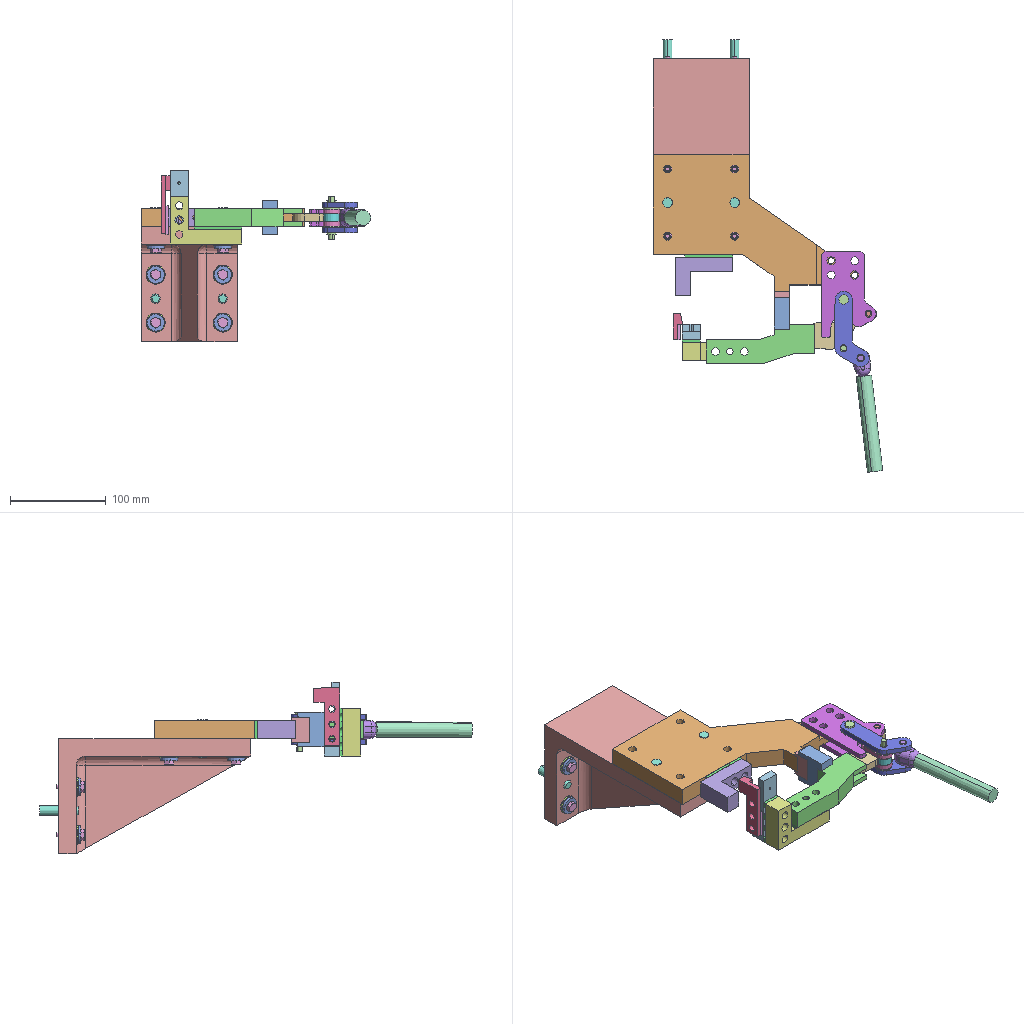Assembly | SolidWorks | 28 different items | 59 placed | box 239 x 451 x 179 mm
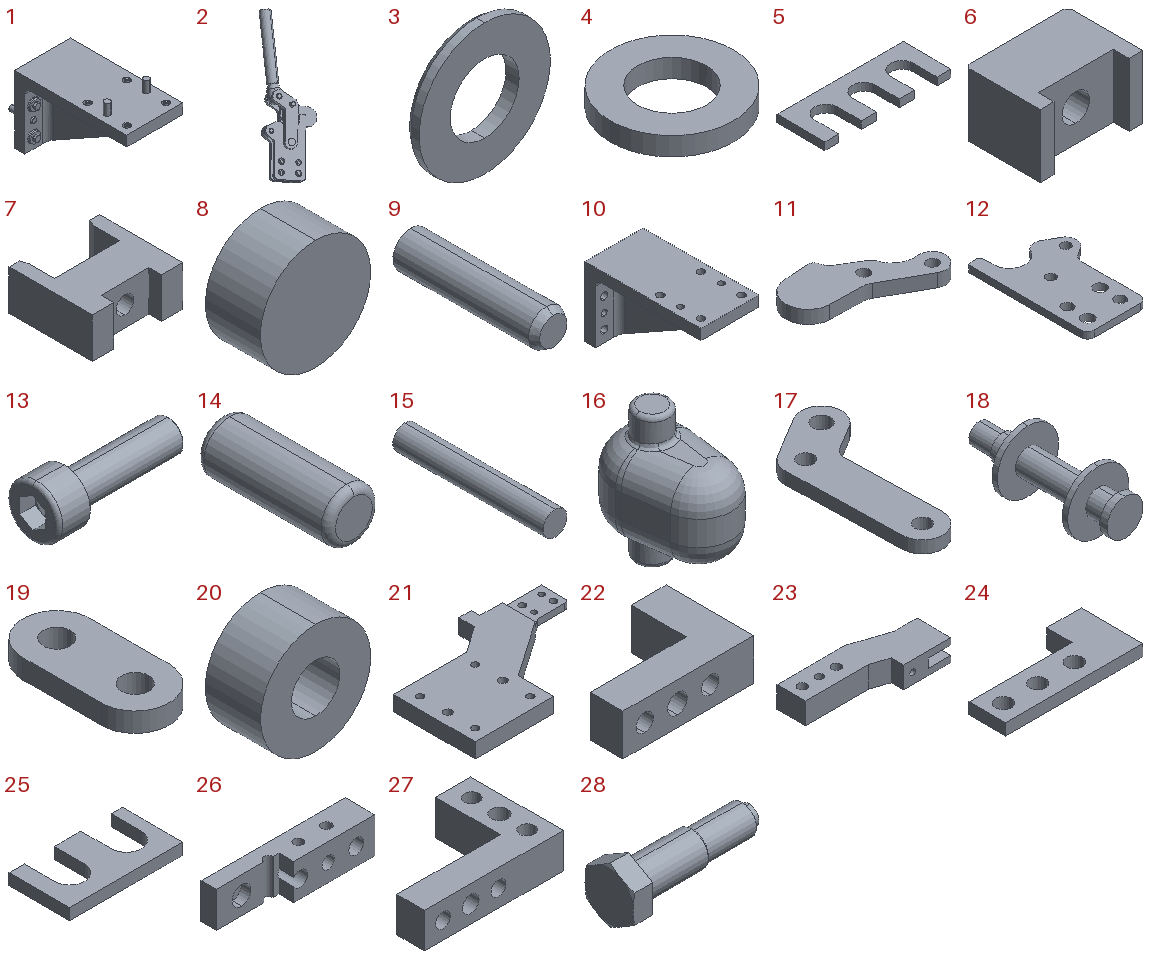Parts list (item | name | quantity | parent item | size | volume | features):
1 | (subassembly) | x1 | - | 100 x 220 x 140 mm | 721947 mm3 | features CompositeCurve 10
2 | (subassembly) | x1 | - | 112.747 x 151.76 x 188.204 mm | 98707 mm3 | features CompositeCurve 3
3 | - | x8 | in 1 | 20 x 2 x 20 mm | 441.839 mm3 | features Chamfer 1, Extrusion 1
4 | - | x8 | in 1 | 18 x 18 x 2.7 mm | 475.009 mm3 | features Extrusion 1
5 | - | x3 | - | 50 x 19 x 3 mm | 1794 mm3 | features Extrusion 1
6 | - | x1 | - | 26 x 19 x 16 mm | 5699 mm3 | features ICE 2, Chamfer 1, Extrusion 1
7 | - | x1 | - | 36 x 33 x 16 mm | 11068 mm3 | features ICE 2, Extrusion 1
8 | - | x1 | - | 10 x 5 x 10 mm | 392.699 mm3 | features Extrusion 1
9 | - | x4 | in 1 | 10 x 40 x 10 mm | 3108 mm3 | features Chamfer 1, Extrusion 1
10 | - | x1 | in 1 | 100 x 200 x 120 mm | 692864 mm3 | features Fillet 2, ICE 2, Extrusion 1, Rib 1
11 | - | x1 | in 2 | 74.927 x 44.837 x 8 mm | 11417 mm3 | features Extrusion 1
12 | - | x2 | in 2 | 56.9 x 90 x 5 mm | 16455 mm3 | features Fillet 2, Extrusion 1
13 | - | x2 | - | 26 x 10 x 10 mm | 958.089 mm3 | features Fillet 2, RevCut 2, Boss 1, Chamfer 1, Cut 1, Extrusion 1, LPattern 1
14 | - | x1 | in 2 | 7 x 18 x 7 mm | 683.885 mm3 | features Extrusion 1, Fillet 1
15 | - | x1 | in 2 | 16 x 100 x 16 mm | 20106 mm3 | features Extrusion 1
16 | - | x1 | in 2 | 19 x 28.3 x 32 mm | 7655 mm3 | features Fillet 3, Extrusion 1, ICE 1
17 | - | x2 | in 2 | 35.738 x 79.423 x 5.4 mm | 7618 mm3 | features Extrusion 1
18 | - | x2 | in 2 | 17 x 40.37 x 17 mm | 2118 mm3 | features ICE 6, Extrusion 1
19 | - | x2 | in 2 | 17.5 x 37.76 x 5 mm | 2591 mm3 | features Extrusion 1
20 | - | x1 | in 2 | 15.9 x 8 x 15.9 mm | 1281 mm3 | features Extrusion 1
21 | - | x1 | - | 220 x 147 x 19 mm | 284001 mm3 | features ICE 4, Extrusion 1, Fillet 1
22 | - | x1 | - | 60 x 40.2 x 19 mm | 22299 mm3 | features Extrusion 1, ICE 1
23 | - | x1 | - | 113 x 41 x 19 mm | 51873 mm3 | features ICE 2, Extrusion 1
24 | - | x1 | - | 60 x 27 x 9.83 mm | 5685 mm3 | features ICE 2, Extrusion 1
25 | - | x1 | - | 30 x 16 x 3 mm | 905.204 mm3 | features Extrusion 1
26 | - | x1 | - | 77 x 16 x 19 mm | 14859 mm3 | features ICE 2, Extrusion 1
27 | - | x1 | - | 75 x 50 x 19 mm | 28429 mm3 | features Extrusion 1, ICE 1
28 | - | x8 | in 1 | 29 x 10 x 11.547 mm | 1165 mm3 | features Boss 2, RevCut 2, Chamfer 1, Cut 1, Extrusion 1, Fillet 1, LPattern 1
Mates (type | each side: item.copy, entity, surface, feature):
In the top assembly
Coincident | 10.1 face plane Boss-Extrude1 | 21.1 face plane Boss-Extrude1
Concentric | 28.1 face cylinder Basebody2 | 21.1 face cylinder Boss-Extrude1
Concentric | 28.2 face cylinder Basebody2 | 21.1 face cylinder Boss-Extrude1
Coincident | 21.1 face plane Cut-Extrude3 | 12.1 face plane Boss-Extrude1
Concentric | 21.1 face cylinder Boss-Extrude1 | 12.2 face cylinder Boss-Extrude1 | 2 times
Coincident | 21.1 face plane Boss-Extrude1 | 5.1 face plane Boss-Extrude1 | 2 times
Concentric | 21.1 face cylinder Cut-Extrude1 | 5.1 face cylinder Boss-Extrude1
Coincident | 22.1 face plane Boss-Extrude1 | 5.1 face plane Boss-Extrude1 | 2 times
Coincident | 21.1 edge | 22.1 face cylinder Cut-Extrude1
Concentric | 6.1 face cylinder Cut-Extrude2 | 13.1 face cylinder BaseBody
Coincident | 6.1 face plane Cut-Extrude1 | 13.1 face plane BaseHead
Concentric | 7.1 face cylinder Cut-Extrude1 | 13.2 face cylinder BaseBody
Coincident | 7.1 face plane Cut-Extrude1 | 13.2 face plane BaseHead
Coincident | 6.1 face plane Boss-Extrude1 | 7.1 face plane Boss-Extrude1 | 3 times
Concentric | 21.1 face cylinder Cut-Extrude2 | 13.1 face cylinder BaseBody
Coincident | 21.1 face plane Boss-Extrude1 | 6.1 face plane Boss-Extrude1 | 2 times
Concentric | 23.1 face cylinder Cut-Extrude2 | 13.2 face cylinder BaseBody
Coincident | 23.1 face plane Boss-Extrude1 | 7.1 face plane Boss-Extrude1 | 2 times
Coincident | 23.1 face plane Boss-Extrude1 | 5.2 face plane Boss-Extrude1
Parallel | 23.1 face plane Boss-Extrude1 | 5.2 face plane Boss-Extrude1
Concentric | 23.1 face cylinder Boss-Extrude1 | 5.2 face cylinder Boss-Extrude1
Coincident | 23.1 face cylinder Boss-Extrude1 | 27.1 edge
Concentric | 23.1 face cylinder Boss-Extrude1 | 27.1 face cylinder Cut-Extrude1
Coincident | 27.1 face plane Boss-Extrude1 | 5.2 face plane Boss-Extrude1
Concentric | 27.1 face cylinder Boss-Extrude1 | 5.3 face cylinder Boss-Extrude1 | 2 times
Coincident | 27.1 face plane Boss-Extrude1 | 5.3 face plane Boss-Extrude1
Concentric | 26.1 face cylinder Cut-Extrude1 | 27.1 face cylinder Boss-Extrude1 | 2 times
Coincident | 26.1 face plane Boss-Extrude1 | 5.3 face plane Boss-Extrude1
Concentric | 26.1 face cylinder Boss-Extrude1 | 25.1 face cylinder Boss-Extrude1 | 2 times
Parallel | 26.1 face plane Boss-Extrude1 | 25.1 face plane Boss-Extrude1
Concentric | 24.1 face cylinder Cut-Extrude2 | 26.1 face cylinder Boss-Extrude1 | 2 times
Coincident | 24.1 face plane Boss-Extrude1 | 25.1 face plane Boss-Extrude1
Concentric | 26.1 face cylinder Cut-Extrude2 | 8.1 face cylinder Boss-Extrude1
Coincident | 26.1 face plane Cut-Extrude2 | 8.1 face plane Boss-Extrude1
In subassembly 2
Concentric | 17.1 face cylinder Boss-Extrude1 | 16.1 face cylinder Boss-Extrude2
Concentric | 16.1 face cylinder Boss-Extrude2 | 17.2 face cylinder Boss-Extrude1
Coincident | 17.1 face plane Boss-Extrude1 | 17.2 face plane Boss-Extrude1
Concentric | 18.1 face cylinder Boss-Extrude4 | 17.2 face cylinder Boss-Extrude1
Concentric | 17.1 face cylinder Boss-Extrude1 | 18.1 face cylinder Boss-Extrude4
Concentric | 18.1 face cylinder Boss-Extrude4 | 19.1 face cylinder Boss-Extrude1
Coincident | 18.1 face plane Boss-Extrude3 | 19.1 face plane Boss-Extrude1
Concentric | 18.1 face cylinder Boss-Extrude4 | 20.1 face cylinder Boss-Extrude1
Coincident | 19.1 face plane Boss-Extrude1 | 20.1 face plane Boss-Extrude1
Concentric | 18.1 face cylinder Boss-Extrude4 | 19.2 face cylinder Boss-Extrude1
Coincident | 18.1 face plane Boss-Extrude5 | 19.2 face plane Boss-Extrude1
Concentric | 19.1 face cylinder Boss-Extrude1 | 19.2 face cylinder Boss-Extrude1
Coincident | 12.3 face plane Boss-Extrude1 | 14.1 face plane Boss-Extrude1
Concentric | 14.1 face cylinder Boss-Extrude1 | 12.4 face cylinder Boss-Extrude1
Coincident | 12.3 face plane Boss-Extrude1 | 12.4 face plane Boss-Extrude1
Coincident | 18.1 face plane Boss-Extrude3 | 17.2 face plane Boss-Extrude1
Coincident | 17.1 face plane Boss-Extrude1 | 18.1 face plane Boss-Extrude5
Concentric | 12.3 face cylinder Boss-Extrude1 | 18.2 face cylinder Boss-Extrude2
Coincident | 12.3 face plane Boss-Extrude1 | 18.2 face plane Boss-Extrude3 | 2 times
Concentric | 17.2 edge | 18.2 face cylinder Boss-Extrude6
Concentric | 14.1 face cylinder Boss-Extrude1 | 11.1 face cylinder Boss-Extrude1
Parallel | 12.3 face plane Boss-Extrude1 | 19.2 face plane Boss-Extrude1
Concentric | 11.1 face cylinder Boss-Extrude1 | 19.2 face cylinder Boss-Extrude1
Coincident | 11.1 face plane Boss-Extrude1 | 19.2 face plane Boss-Extrude1
Coincident | 16.1 face plane Boss-Extrude2 | 17.2 face plane Boss-Extrude1
Coincident | 17.1 face plane Boss-Extrude1 | 18.2 face plane Boss-Extrude3
Coincident | 11.1 face plane Boss-Extrude1 | 12.4 face plane Boss-Extrude1
Lock | 15.1 select_type:0 | 16.1 select_type:0
In subassembly 1
Concentric | 10.2 face cylinder Cut-Extrude2 | 3.1 face cylinder Boss-Extrude1
Coincident | 10.2 face plane Boss-Extrude1 | 3.1 face plane Boss-Extrude1
Coincident | 4.1 face plane Boss-Extrude1 | 3.1 face plane Boss-Extrude1
Concentric | 4.1 face cylinder Boss-Extrude1 | 3.1 face cylinder Boss-Extrude1
Coincident | 10.2 face plane Boss-Extrude1 | 3.2 face plane Boss-Extrude1
Concentric | 10.2 face cylinder Cut-Extrude2 | 3.2 face cylinder Boss-Extrude1
Coincident | 3.2 face plane Boss-Extrude1 | 4.2 face plane Boss-Extrude1
Concentric | 3.2 face cylinder Boss-Extrude1 | 4.2 face cylinder Boss-Extrude1
Coincident | 10.2 face plane Boss-Extrude1 | 3.3 face plane Boss-Extrude1
Concentric | 10.2 face cylinder Cut-Extrude2 | 3.3 face cylinder Boss-Extrude1
Concentric | 4.3 face cylinder Boss-Extrude1 | 3.3 face cylinder Boss-Extrude1
Coincident | 4.3 face plane Boss-Extrude1 | 3.3 face plane Boss-Extrude1
Coincident | 4.4 face plane Boss-Extrude1 | 3.4 face plane Boss-Extrude1
Concentric | 4.4 face cylinder Boss-Extrude1 | 3.4 face cylinder Boss-Extrude1
Coincident | 10.2 face plane Boss-Extrude1 | 3.4 face plane Boss-Extrude1
Concentric | 10.2 face cylinder Cut-Extrude2 | 4.4 face cylinder Boss-Extrude1
Coincident | 4.5 face plane Boss-Extrude1 | 3.5 face plane Boss-Extrude1
Concentric | 4.5 face cylinder Boss-Extrude1 | 3.5 face cylinder Boss-Extrude1
Concentric | 10.2 face cylinder Cut-Extrude3 | 4.5 face cylinder Boss-Extrude1
Concentric | 10.2 face cylinder Cut-Extrude3 | 3.5 edge
Coincident | 10.2 face plane Boss-Extrude1 | 3.5 face plane Boss-Extrude1
Coincident | 4.6 face plane Boss-Extrude1 | 3.6 face plane Boss-Extrude1
Concentric | 4.6 face cylinder Boss-Extrude1 | 3.6 face cylinder Boss-Extrude1
Coincident | 10.2 face plane Boss-Extrude1 | 3.6 face plane Boss-Extrude1
Concentric | 10.2 face cylinder Cut-Extrude3 | 4.6 face cylinder Boss-Extrude1
Coincident | 4.7 face plane Boss-Extrude1 | 3.7 face plane Boss-Extrude1
Concentric | 4.7 face cylinder Boss-Extrude1 | 3.7 face cylinder Boss-Extrude1
Concentric | 10.2 face cylinder Cut-Extrude3 | 4.7 face cylinder Boss-Extrude1
Coincident | 10.2 face plane Boss-Extrude1 | 3.7 face plane Boss-Extrude1
Coincident | 4.8 face plane Boss-Extrude1 | 3.8 face plane Boss-Extrude1
Concentric | 4.8 face cylinder Boss-Extrude1 | 3.8 face cylinder Boss-Extrude1
Concentric | 10.2 face cylinder Cut-Extrude3 | 4.8 face cylinder Boss-Extrude1
Coincident | 10.2 face plane Boss-Extrude1 | 3.8 face plane Boss-Extrude1
Concentric | 10.2 face cylinder Cut-Extrude2 | 28.3 face cylinder Basebody1
Coincident | 4.1 face plane Boss-Extrude1 | 28.3 face plane BaseHead
Concentric | 10.2 face cylinder Cut-Extrude2 | 28.4 face cylinder Basebody2
Coincident | 4.2 face plane Boss-Extrude1 | 28.4 face plane BaseHead
Concentric | 4.4 face cylinder Boss-Extrude1 | 28.5 face cylinder Basebody2
Coincident | 4.4 face plane Boss-Extrude1 | 28.5 face plane BaseHead
Concentric | 4.3 face cylinder Boss-Extrude1 | 28.6 face cylinder Basebody2
Coincident | 4.3 face plane Boss-Extrude1 | 28.6 face plane BaseHead
Concentric | 4.5 face cylinder Boss-Extrude1 | 28.7 face cylinder Basebody2
Coincident | 4.5 face plane Boss-Extrude1 | 28.7 face plane BaseHead
Concentric | 4.6 face cylinder Boss-Extrude1 | 28.8 face cylinder Basebody2
Coincident | 4.6 face plane Boss-Extrude1 | 28.8 face plane BaseHead
Concentric | 4.7 face cylinder Boss-Extrude1 | 28.9 face cylinder Basebody2
Coincident | 4.7 face plane Boss-Extrude1 | 28.9 face plane BaseHead
Concentric | 4.8 face cylinder Boss-Extrude1 | 28.10 face cylinder Basebody2
Coincident | 4.8 face plane Boss-Extrude1 | 28.10 face plane BaseHead
Concentric | 10.2 face cylinder Cut-Extrude2 | 9.1 face cylinder Boss-Extrude1
Coincident | 10.2 edge | 9.1 edge
Concentric | 10.2 face cylinder Cut-Extrude2 | 9.2 face cylinder Boss-Extrude1
Coincident | 10.2 edge | 9.2 edge
Concentric | 10.2 face cylinder Cut-Extrude3 | 9.3 face cylinder Boss-Extrude1
Coincident | 10.2 edge | 9.3 edge
Concentric | 10.2 face cylinder Cut-Extrude3 | 9.4 face cylinder Boss-Extrude1
Coincident | 10.2 edge | 9.4 edge